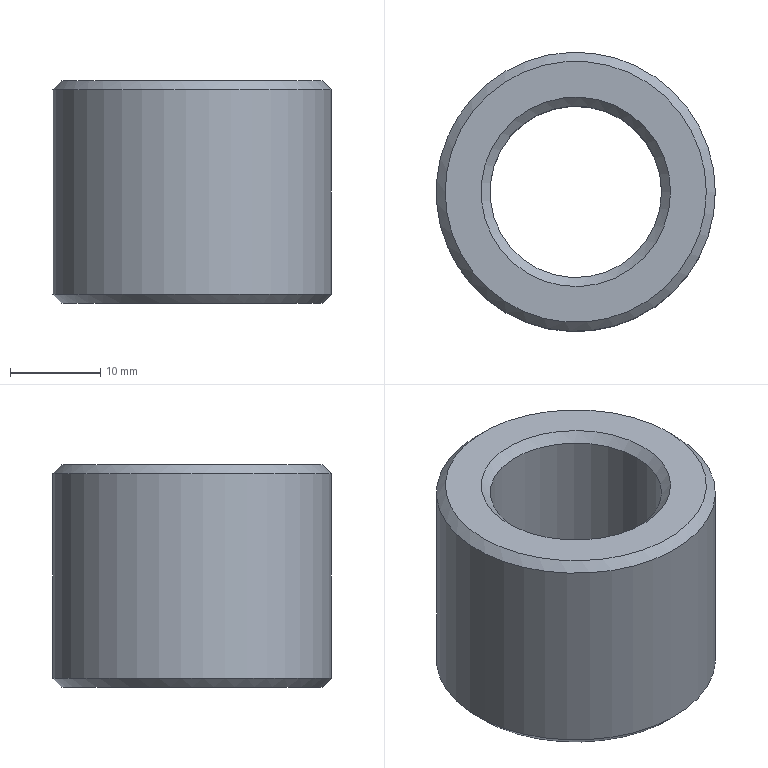Part | NX | features solid 2 | 1 solid | 8 faces | box 31 x 31 x 24.675 mm | volume 11434 mm3 | cone 4 | cylinder 2 | plane 2 | commonest cylinder face diameters 19.05 x1 31 x1
STEP:
#1=CARTESIAN_POINT('',(15.5,0.,1.));
#2=VERTEX_POINT('',#1);
#3=CARTESIAN_POINT('',(0.,0.,1.));
#4=DIRECTION('',(0.,0.,1.));
#5=DIRECTION('',(1.,0.,0.));
#6=AXIS2_PLACEMENT_3D('',#3,#4,#5);
#7=CIRCLE('',#6,15.5);
#8=EDGE_CURVE('',#2,#2,#7,.T.);
#9=ORIENTED_EDGE('',*,*,#8,.T.);
#10=EDGE_LOOP('',(#9));
#11=FACE_BOUND('',#10,.T.);
#12=CARTESIAN_POINT('',(15.5,0.,23.675));
#13=VERTEX_POINT('',#12);
#14=CARTESIAN_POINT('',(0.,0.,23.675));
#15=DIRECTION('',(0.,0.,1.));
#16=DIRECTION('',(1.,0.,0.));
#17=AXIS2_PLACEMENT_3D('',#14,#15,#16);
#18=CIRCLE('',#17,15.5);
#19=EDGE_CURVE('',#13,#13,#18,.F.);
#20=ORIENTED_EDGE('',*,*,#19,.T.);
#21=EDGE_LOOP('',(#20));
#22=FACE_BOUND('',#21,.T.);
#23=CARTESIAN_POINT('',(0.,0.,24.675));
#24=DIRECTION('',(0.,0.,-1.));
#25=DIRECTION('',(-1.,0.,0.));
#26=AXIS2_PLACEMENT_3D('',#23,#24,#25);
#27=CYLINDRICAL_SURFACE('',#26,15.5);
#28=ADVANCED_FACE('',(#11,#22),#27,.T.);
#29=CARTESIAN_POINT('',(9.525,0.,1.));
#30=VERTEX_POINT('',#29);
#31=CARTESIAN_POINT('',(0.,0.,1.));
#32=DIRECTION('',(0.,0.,1.));
#33=DIRECTION('',(1.,0.,0.));
#34=AXIS2_PLACEMENT_3D('',#31,#32,#33);
#35=CIRCLE('',#34,9.525);
#36=EDGE_CURVE('',#30,#30,#35,.F.);
#37=ORIENTED_EDGE('',*,*,#36,.T.);
#38=EDGE_LOOP('',(#37));
#39=FACE_BOUND('',#38,.T.);
#40=CARTESIAN_POINT('',(9.525,0.,23.675));
#41=VERTEX_POINT('',#40);
#42=CARTESIAN_POINT('',(0.,0.,23.675));
#43=DIRECTION('',(0.,0.,1.));
#44=DIRECTION('',(1.,0.,0.));
#45=AXIS2_PLACEMENT_3D('',#42,#43,#44);
#46=CIRCLE('',#45,9.525);
#47=EDGE_CURVE('',#41,#41,#46,.T.);
#48=ORIENTED_EDGE('',*,*,#47,.T.);
#49=EDGE_LOOP('',(#48));
#50=FACE_BOUND('',#49,.T.);
#51=CARTESIAN_POINT('',(0.,0.,24.675));
#52=DIRECTION('',(0.,0.,-1.));
#53=DIRECTION('',(-1.,0.,0.));
#54=AXIS2_PLACEMENT_3D('',#51,#52,#53);
#55=CYLINDRICAL_SURFACE('',#54,9.525);
#56=ADVANCED_FACE('',(#39,#50),#55,.F.);
#57=CARTESIAN_POINT('',(10.525,0.,24.675));
#58=VERTEX_POINT('',#57);
#59=CARTESIAN_POINT('',(0.,0.,24.675));
#60=DIRECTION('',(0.,0.,1.));
#61=DIRECTION('',(1.,0.,0.));
#62=AXIS2_PLACEMENT_3D('',#59,#60,#61);
#63=CIRCLE('',#62,10.525);
#64=EDGE_CURVE('',#58,#58,#63,.F.);
#65=ORIENTED_EDGE('',*,*,#64,.T.);
#66=EDGE_LOOP('',(#65));
#67=FACE_BOUND('',#66,.T.);
#68=CARTESIAN_POINT('',(14.5,0.,24.675));
#69=VERTEX_POINT('',#68);
#70=CARTESIAN_POINT('',(0.,0.,24.675));
#71=DIRECTION('',(0.,0.,1.));
#72=DIRECTION('',(1.,0.,0.));
#73=AXIS2_PLACEMENT_3D('',#70,#71,#72);
#74=CIRCLE('',#73,14.5);
#75=EDGE_CURVE('',#69,#69,#74,.T.);
#76=ORIENTED_EDGE('',*,*,#75,.T.);
#77=EDGE_LOOP('',(#76));
#78=FACE_BOUND('',#77,.T.);
#79=CARTESIAN_POINT('',(0.,0.,24.675));
#80=DIRECTION('',(0.,0.,1.));
#81=DIRECTION('',(1.,0.,0.));
#82=AXIS2_PLACEMENT_3D('',#79,#80,#81);
#83=PLANE('',#82);
#84=ADVANCED_FACE('',(#67,#78),#83,.T.);
#85=CARTESIAN_POINT('',(10.525,0.,0.));
#86=VERTEX_POINT('',#85);
#87=CARTESIAN_POINT('',(0.,0.,0.));
#88=DIRECTION('',(0.,0.,1.));
#89=DIRECTION('',(1.,0.,0.));
#90=AXIS2_PLACEMENT_3D('',#87,#88,#89);
#91=CIRCLE('',#90,10.525);
#92=EDGE_CURVE('',#86,#86,#91,.T.);
#93=ORIENTED_EDGE('',*,*,#92,.T.);
#94=EDGE_LOOP('',(#93));
#95=FACE_BOUND('',#94,.T.);
#96=CARTESIAN_POINT('',(14.5,0.,0.));
#97=VERTEX_POINT('',#96);
#98=CARTESIAN_POINT('',(0.,0.,0.));
#99=DIRECTION('',(0.,0.,1.));
#100=DIRECTION('',(1.,0.,0.));
#101=AXIS2_PLACEMENT_3D('',#98,#99,#100);
#102=CIRCLE('',#101,14.5);
#103=EDGE_CURVE('',#97,#97,#102,.F.);
#104=ORIENTED_EDGE('',*,*,#103,.T.);
#105=EDGE_LOOP('',(#104));
#106=FACE_BOUND('',#105,.T.);
#107=CARTESIAN_POINT('',(0.,0.,0.));
#108=DIRECTION('',(0.,0.,1.));
#109=DIRECTION('',(1.,0.,0.));
#110=AXIS2_PLACEMENT_3D('',#107,#108,#109);
#111=PLANE('',#110);
#112=ADVANCED_FACE('',(#95,#106),#111,.F.);
#113=ORIENTED_EDGE('',*,*,#36,.F.);
#114=EDGE_LOOP('',(#113));
#115=FACE_BOUND('',#114,.T.);
#116=ORIENTED_EDGE('',*,*,#92,.F.);
#117=EDGE_LOOP('',(#116));
#118=FACE_BOUND('',#117,.T.);
#119=CARTESIAN_POINT('',(0.,0.,0.));
#120=DIRECTION('',(0.,0.,-1.));
#121=DIRECTION('',(-1.,0.,0.));
#122=AXIS2_PLACEMENT_3D('',#119,#120,#121);
#123=CONICAL_SURFACE('',#122,10.525,0.7854);
#124=ADVANCED_FACE('',(#115,#118),#123,.F.);
#125=ORIENTED_EDGE('',*,*,#103,.F.);
#126=EDGE_LOOP('',(#125));
#127=FACE_BOUND('',#126,.T.);
#128=ORIENTED_EDGE('',*,*,#8,.F.);
#129=EDGE_LOOP('',(#128));
#130=FACE_BOUND('',#129,.T.);
#131=CARTESIAN_POINT('',(0.,0.,1.));
#132=DIRECTION('',(0.,0.,1.));
#133=DIRECTION('',(1.,0.,0.));
#134=AXIS2_PLACEMENT_3D('',#131,#132,#133);
#135=CONICAL_SURFACE('',#134,15.5,0.7854);
#136=ADVANCED_FACE('',(#127,#130),#135,.T.);
#137=ORIENTED_EDGE('',*,*,#64,.F.);
#138=EDGE_LOOP('',(#137));
#139=FACE_BOUND('',#138,.T.);
#140=ORIENTED_EDGE('',*,*,#47,.F.);
#141=EDGE_LOOP('',(#140));
#142=FACE_BOUND('',#141,.T.);
#143=CARTESIAN_POINT('',(0.,0.,23.675));
#144=DIRECTION('',(0.,0.,1.));
#145=DIRECTION('',(1.,0.,0.));
#146=AXIS2_PLACEMENT_3D('',#143,#144,#145);
#147=CONICAL_SURFACE('',#146,9.525,0.7854);
#148=ADVANCED_FACE('',(#139,#142),#147,.F.);
#149=ORIENTED_EDGE('',*,*,#19,.F.);
#150=EDGE_LOOP('',(#149));
#151=FACE_BOUND('',#150,.T.);
#152=ORIENTED_EDGE('',*,*,#75,.F.);
#153=EDGE_LOOP('',(#152));
#154=FACE_BOUND('',#153,.T.);
#155=CARTESIAN_POINT('',(0.,0.,24.675));
#156=DIRECTION('',(0.,0.,-1.));
#157=DIRECTION('',(-1.,0.,0.));
#158=AXIS2_PLACEMENT_3D('',#155,#156,#157);
#159=CONICAL_SURFACE('',#158,14.5,0.7854);
#160=ADVANCED_FACE('',(#151,#154),#159,.T.);
#161=CLOSED_SHELL('',(#28,#56,#84,#112,#124,#136,#148,#160));
#162=MANIFOLD_SOLID_BREP('',#161);
#163=(LENGTH_UNIT()NAMED_UNIT(*)SI_UNIT(.MILLI.,.METRE.));
#164=UNCERTAINTY_MEASURE_WITH_UNIT(LENGTH_MEASURE(0.00001),#163,'','');
#165=(NAMED_UNIT(*)PLANE_ANGLE_UNIT()SI_UNIT($,.RADIAN.));
#166=(NAMED_UNIT(*)SI_UNIT($,.STERADIAN.)SOLID_ANGLE_UNIT());
#167=(GEOMETRIC_REPRESENTATION_CONTEXT(3)GLOBAL_UNCERTAINTY_ASSIGNED_CONTEXT((#164))GLOBAL_UNIT_ASSIGNED_CONTEXT((#163,#165,#166))REPRESENTATION_CONTEXT('',''));
#168=ADVANCED_BREP_SHAPE_REPRESENTATION('',(#162),#167);